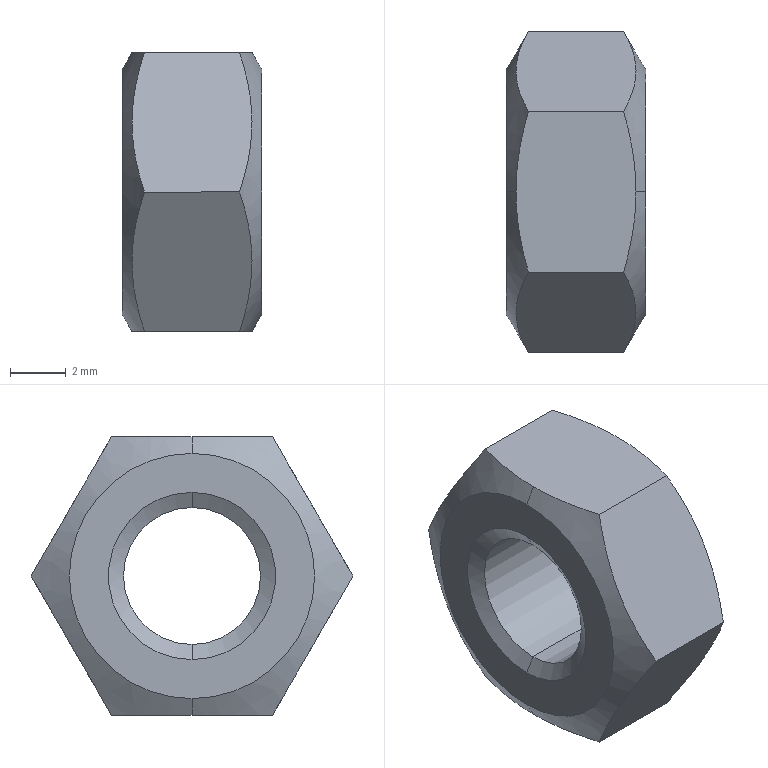Part | STEP file | DIN 934 - M6 x 1 | 1 solid | 18 faces | box 5 x 11.547 x 10 mm | volume 321.226 mm3 | cone 8 | plane 8 | cylinder 2 | commonest cylinder face diameters 4.917 x2